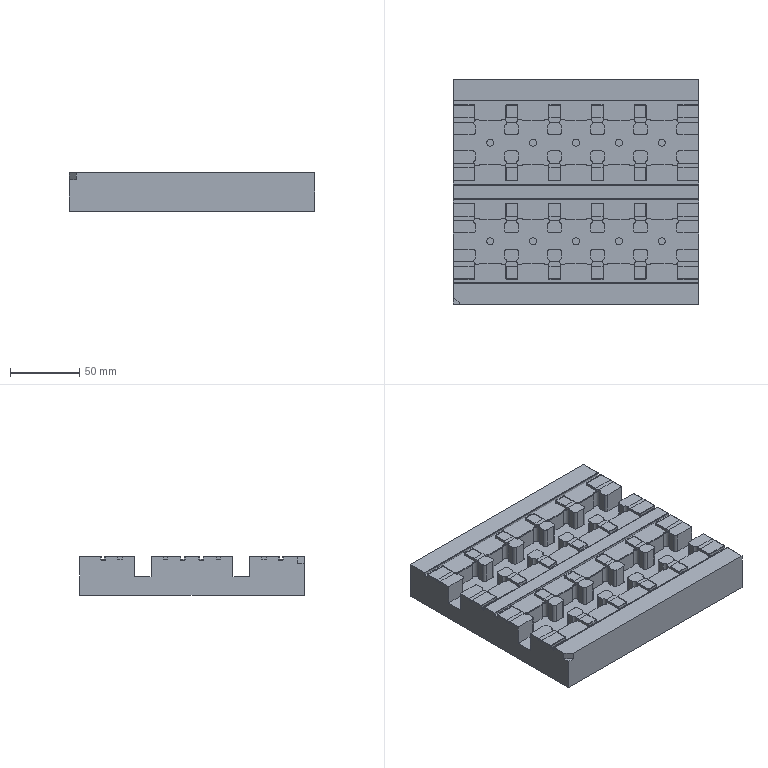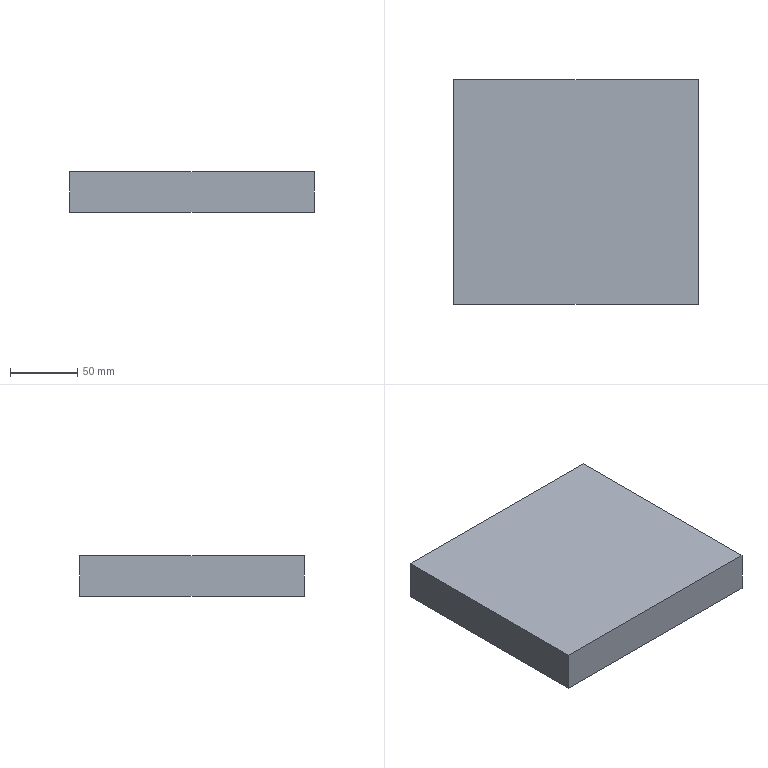CAM job | NX | 3-axis milling, drilling | part box 177 x 162 x 28 mm | stock box 182 x 167 x 30 mm
Tools:
number,name,description,diameter,corner_radius,flute_length,length,flutes
4,D3,平底铣刀-粗,3.0,0.0,50.0,75.0,2
5,D4,平底铣刀-粗,4.0,0.0,50.0,75.0,2
10,D10,平底铣刀-粗,10.0,0.0,50.0,75.0,2
13,D3-J,平底铣刀-精,3.0,0.0,50.0,75.0,2
14,D4-J,平底铣刀-精,4.0,0.0,50.0,75.0,2
7,D6-J,平底铣刀-精,6.0,0.0,50.0,75.0,2
11,D10-J,平底铣刀-精,10.0,0.0,50.0,75.0,2
2,D17R0.8FLYCUTTER,圆鼻刀-粗,17.0,0.8,50.0,75.0,2
1,D6CHAMFERMILL,倒角刀,6.0,0.0,3.0,75.0,2
17,C6SPOTDRILL,倒角刀,6.0,0.0,3.0,3.0,2
15,ZT4.5,钻头,4.5,0.0,35.0,50.0,2
3,ZT5.1,钻头,5.1,0.0,35.0,50.0,2
Operations:
program,operation,operation_type,tool,method,geometry_group,spindle_rpm,surface_speed,feed_per_tooth,feed_cut,feed_plunge,cut_length_mm,path_length_mm,cut_time_min,machine_time_min
FIXTURE2-B,TOPFACE_3,FaceMilling,D17R0.8FLYCUTTER,LAYERROUGH-DEPTHK-STEPG,W-D,2000.0,106.814,0.625,2500.0,100.0,22876.873,23865.921,9.151,9.25
FIXTURE2-B,SPOTDRILL_3_COPY,Operation,C6SPOTDRILL,METHOD,W-D,1500.0,28.274,0.0167,50.0,0.0,72.0,886.249,1.44,1.521
FIXTURE2-B,SPOTDRILL_3_COPY_COPY,Operation,ZT4.5,METHOD,W-D,1500.0,28.274,0.0167,50.0,0.0,620.0,1982.249,12.4,12.536
FIXTURE2-B,FLOORWALLLAYERROUGH-MID_COPY,VolumeBased25DMillingOperation,D10,LAYERROUGH-DEPTHK-STEPG,W-D,3000.0,94.245,0.3333,2000.0,100.0,102428.418,102629.823,51.214,51.234
FIXTURE2-B,FLOORWALLLAYERROUGH-MID_COPY_COPY,VolumeBased25DMillingOperation,D10,LAYERROUGH-DEPTHK-STEPG,W-D,3000.0,94.245,0.3333,2000.0,100.0,22675.342,24246.354,11.338,11.495
FIXTURE2-B,ZLEVELZIGZAGROUGH-MID_2,ZLevelMilling,D10,LAYERROUGH-DEPTHK-STEPG,W-D,3000.0,94.248,0.5,3000.0,100.0,377.421,417.221,0.1258,0.1754
FIXTURE2-B,CORNERCLEARD4_COPY_COPY,ZLevelMilling,D4,METHOD,W-D,4000.0,50.266,0.1875,1500.0,80.0,24212.13,25204.509,16.148,16.247
FIXTURE2-B,CORNERCLEARD4_COPY_1,ZLevelMilling,D4,METHOD,W-D,4000.0,50.266,0.25,2000.0,80.0,51763.623,54082.188,25.893,26.125
FIXTURE2-B,ZLEVELFINISH-MID_COPY_COPY_COPY,ZLevelMilling,D4,SIDEEDGEFINISH-DEPTHK-STEPG,W-D,4000.0,50.266,0.125,1000.0,100.0,3597.693,5771.391,3.598,3.815
FIXTURE2-B,WIREZIGZAGROUGH-MID_COPY_COPY_2,PlanarMilling,D3,LAYERROUGH-DEPTHK-STEPG,W-D,5000.0,47.124,0.15,1500.0,100.0,33840.0,34109.74,22.56,22.587
FIXTURE2-B,FLOORWALLFINISHSIDE-MID-SELECTBOTTOMFACE_COPY_1,VolumeBased25DMillingOperation,D3,SIDEEDGEFINISH-DEPTHK-STEPG,W-D,5000.0,47.124,0.1,1000.0,100.0,974.846,2361.672,0.9748,1.113
FIXTURE2-B,SPOTDRILL_3,Operation,C6SPOTDRILL,METHOD,W-D,1500.0,28.274,0.02,60.0,0.0,18.0,423.336,0.3,0.3405
FIXTURE2-B,DRILL_2,Operation,ZT5.1,METHOD,W-D,1200.0,18.85,0.05,120.0,0.0,130.25,647.836,1.085,1.137
FIXTURE2-B,TOPFACE_4,FaceMilling,D10-J,SIDEEDGEFINISH-DEPTHK-STEPG,W-D,3000.0,94.248,0.1667,1000.0,100.0,6534.171,6560.171,6.534,6.537
FIXTURE2-B,BOTTOMFINISH_4,VolumeBased25DMillingOperation,D4-J,METHOD,W-D,4000.0,75.398,0.125,1000.0,90.0,3179.036,3366.736,3.18,3.199
FIXTURE2-B,BOTTOMFINISH_5,VolumeBased25DMillingOperation,D3-J,METHOD,W-D,4000.0,75.398,0.125,1000.0,90.0,3398.438,4783.187,3.409,3.547
FIXTURE2-B,CHAMFER_4,SurfaceContour,D6CHAMFERMILL,METHOD,W-D,3000.0,942.0,0.1667,1000.0,100.0,3931.713,8495.775,3.932,4.388
FIXTURE2-B,CHAMFERMILL_2,PlanarMilling,D6CHAMFERMILL,METHOD,W-D,4000.0,75.398,0.0625,500.0,100.0,182.493,1112.496,0.365,0.458
FIXTURE2-B,BOTTOMSIDEFINISH_7,VolumeBased25DMillingOperation,D6-J,METHOD,W-D,4000.0,75.398,0.1,800.0,90.0,12.871,51.871,0.0163,0.0202
FIXTURE2-B,ZLEVELFINISH-MID_COPY_COPY_1,ZLevelMilling,D4-J,SIDEEDGEFINISH-DEPTHK-STEPG,W-D,4000.0,50.266,0.0875,700.0,100.0,3597.084,5771.477,5.139,5.356
FIXTURE2-B,FLOORWALLFINISHSIDE-MID-SELECTBOTTOMFACE_COPY,VolumeBased25DMillingOperation,D3-J,SIDEEDGEFINISH-DEPTHK-STEPG,W-D,4500.0,42.411,0.0778,700.0,100.0,1690.033,2518.973,2.414,2.497
FIXTURE2-A,Z0.5FACEMILLAUTOROUGHD10_COPY,FaceMilling,D17R0.8FLYCUTTER,LAYERROUGH-DEPTHK-STEPG,W-C,2000.0,106.814,0.75,3000.0,100.0,6579.882,6836.024,2.193,2.219
FIXTURE2-A,FLOORWALLHELICALROUGH-MIDD17R0.8-0.5_COPY,VolumeBased25DMillingOperation,D17R0.8FLYCUTTER,LAYERROUGH-DEPTHK-STEPG,W-C,2000.0,106.814,0.75,3000.0,100.0,71821.557,71948.557,23.941,23.953
FIXTURE2-A,PROFILESEMIFINISHD10_COPY,VolumeBased25DMillingOperation,D10,METHOD,W-C,3000.0,942.0,0.25,1500.0,100.0,4285.508,4501.859,2.857,2.879
FIXTURE2-A,FACEMILLAUTOFINISHD10-J_COPY,FaceMilling,D10-J,SIDEEDGEFINISH-DEPTHK-STEPG,W-C,3000.0,94.248,0.1667,1000.0,100.0,6548.171,6644.171,6.548,6.558
FIXTURE2-A,CHAMFER_2_COPY,SurfaceContour,D6CHAMFERMILL,METHOD,W-C,3000.0,942.0,0.1667,1000.0,100.0,695.315,791.116,0.6953,0.7049
FIXTURE2-A,PROFILEFINISHD10_COPY,VolumeBased25DMillingOperation,D10-J,METHOD,W-C,3000.0,942.0,0.1667,1000.0,100.0,4291.034,4707.063,4.291,4.333
FIXTURE1-A,Z0.5FACEMILLAUTOROUGHD10,FaceMilling,D17R0.8FLYCUTTER,LAYERROUGH-DEPTHK-STEPG,W-A,2000.0,106.814,0.75,3000.0,100.0,6579.882,6766.024,2.193,2.212
FIXTURE1-A,FLOORWALLHELICALROUGH-MIDD17R0.8-0.5,VolumeBased25DMillingOperation,D17R0.8FLYCUTTER,LAYERROUGH-DEPTHK-STEPG,W-A,2000.0,106.814,0.75,3000.0,100.0,71821.557,71878.557,23.941,23.946
FIXTURE1-A,PROFILESEMIFINISHD10,VolumeBased25DMillingOperation,D10,METHOD,W-A,3000.0,942.0,0.25,1500.0,100.0,4285.508,4431.859,2.857,2.872
FIXTURE1-A,FACEMILLAUTOFINISHD10-J,FaceMilling,D10-J,SIDEEDGEFINISH-DEPTHK-STEPG,W-A,3000.0,94.248,0.1667,1000.0,100.0,6548.171,6574.171,6.548,6.551
FIXTURE1-A,CHAMFER_2,SurfaceContour,D6CHAMFERMILL,METHOD,W-A,3000.0,942.0,0.1667,1000.0,100.0,695.315,721.116,0.6953,0.6979
FIXTURE1-A,PROFILEFINISHD10,VolumeBased25DMillingOperation,D10-J,METHOD,W-A,3000.0,942.0,0.1667,1000.0,100.0,4291.034,4497.063,4.291,4.312
FIXTURE1-B,TOPFACE,FaceMilling,D17R0.8FLYCUTTER,LAYERROUGH-DEPTHK-STEPG,W-B,2000.0,106.814,0.625,2500.0,100.0,26144.998,27294.586,10.458,10.573
FIXTURE1-B,SPOTDRILL_COPY,Operation,C6SPOTDRILL,METHOD,W-B,1500.0,28.274,0.0167,50.0,0.0,72.0,886.249,1.44,1.521
FIXTURE1-B,SPOTDRILL_COPY_COPY,Operation,ZT4.5,METHOD,W-B,1000.0,14.137,0.025,50.0,0.0,620.0,1982.249,12.4,12.536
FIXTURE1-B,FLOORWALLROUGH_1,VolumeBased25DMillingOperation,D10,METHOD,W-B,3000.0,94.248,0.3333,2000.0,100.0,44087.507,44726.094,22.044,22.108
FIXTURE1-B,FLOORWALLROUGH_2,VolumeBased25DMillingOperation,D10,METHOD,W-B,3000.0,94.248,0.3333,2000.0,100.0,49649.285,50280.707,24.825,24.888
FIXTURE1-B,FLOORWALLROUGH_3,VolumeBased25DMillingOperation,D10,METHOD,W-B,3000.0,94.248,0.3333,2000.0,100.0,13456.717,16202.684,6.728,7.003
FIXTURE1-B,ZLEVELZIGZAGROUGH-MID_1,ZLevelMilling,D10,LAYERROUGH-DEPTHK-STEPG,W-B,3000.0,94.248,0.5,3000.0,100.0,355.88,395.295,0.1186,0.1663
FIXTURE1-B,CORNERCLEARD4_COPY,ZLevelMilling,D4,METHOD,W-B,4000.0,50.266,0.1875,1500.0,80.0,17414.063,19177.07,11.624,11.8
FIXTURE1-B,CORNERCLEARD4,ZLevelMilling,D4,METHOD,W-B,4000.0,50.266,0.25,2000.0,80.0,58214.908,61078.134,29.118,29.404
FIXTURE1-B,ZLEVELFINISH-MID_COPY_COPY,ZLevelMilling,D4,SIDEEDGEFINISH-DEPTHK-STEPG,W-B,4000.0,50.266,0.125,1000.0,100.0,3597.693,5771.391,3.598,3.815
FIXTURE1-B,WIREZIGZAGROUGH-MID_COPY,PlanarMilling,D3,LAYERROUGH-DEPTHK-STEPG,W-B,5000.0,47.124,0.15,1500.0,100.0,22560.0,23276.242,15.04,15.112
FIXTURE1-B,WIREZIGZAGROUGH-MID_COPY_COPY,PlanarMilling,D3,LAYERROUGH-DEPTHK-STEPG,W-B,5000.0,47.124,0.1,1000.0,100.0,22560.0,22798.24,22.56,22.584
FIXTURE1-B,FLOORWALLFINISHSIDE-MID-SELECTBOTTOMFACE_COPY_1_COPY,VolumeBased25DMillingOperation,D3,SIDEEDGEFINISH-DEPTHK-STEPG,W-B,5000.0,47.124,0.1,1000.0,100.0,1388.837,2598.641,1.389,1.51
FIXTURE1-B,TOPFACE_2,FaceMilling,D10-J,SIDEEDGEFINISH-DEPTHK-STEPG,W-B,3000.0,94.248,0.1667,1000.0,100.0,6534.171,6560.171,6.534,6.537
FIXTURE1-B,SPOTDRILL,Operation,C6SPOTDRILL,METHOD,W-B,1500.0,28.274,0.0167,50.0,0.0,9.0,205.565,0.18,0.1997
FIXTURE1-B,SPOTDRILL_2,Operation,C6SPOTDRILL,METHOD,W-B,1500.0,28.274,0.0167,50.0,0.0,9.0,205.565,0.18,0.1997
FIXTURE1-B,DRILL,Operation,ZT5.1,METHOD,W-B,1000.0,15.708,0.025,50.0,0.0,127.75,643.336,2.555,2.607
FIXTURE1-B,BOTTOMFINISH_1,VolumeBased25DMillingOperation,D4-J,METHOD,W-B,4000.0,75.398,0.125,1000.0,90.0,1589.518,1647.518,1.59,1.596
FIXTURE1-B,BOTTOMFINISH_2,VolumeBased25DMillingOperation,D4-J,METHOD,W-B,4000.0,75.398,0.125,1000.0,90.0,1589.518,1647.518,1.59,1.596
FIXTURE1-B,BOTTOMFINISH_3,VolumeBased25DMillingOperation,D3-J,METHOD,W-B,4000.0,75.398,0.125,1000.0,90.0,3723.44,5073.172,3.734,3.869
FIXTURE1-B,CHAMFER_3,SurfaceContour,D6CHAMFERMILL,METHOD,W-B,3000.0,942.0,0.1667,1000.0,100.0,4836.795,10978.962,4.837,5.451
FIXTURE1-B,CHAMFERMILL_1,PlanarMilling,D6CHAMFERMILL,METHOD,W-B,4000.0,75.398,0.0375,300.0,100.0,171.372,1108.701,0.5712,0.665
FIXTURE1-B,BOTTOMSIDEFINISH_6,VolumeBased25DMillingOperation,D6-J,METHOD,W-B,5000.0,62.832,0.08,800.0,90.0,12.871,51.861,0.0163,0.0202
FIXTURE1-B,ZLEVELFINISH-MID_COPY,ZLevelMilling,D4-J,SIDEEDGEFINISH-DEPTHK-STEPG,W-B,4000.0,50.266,0.075,600.0,100.0,3597.084,5771.477,5.995,6.213
FIXTURE1-B,FLOORWALLFINISHSIDE-MID-SELECTBOTTOMFACE_COPY_2,VolumeBased25DMillingOperation,D3-J,SIDEEDGEFINISH-DEPTHK-STEPG,W-B,5000.0,47.124,0.06,600.0,100.0,2726.689,3949.296,4.545,4.667